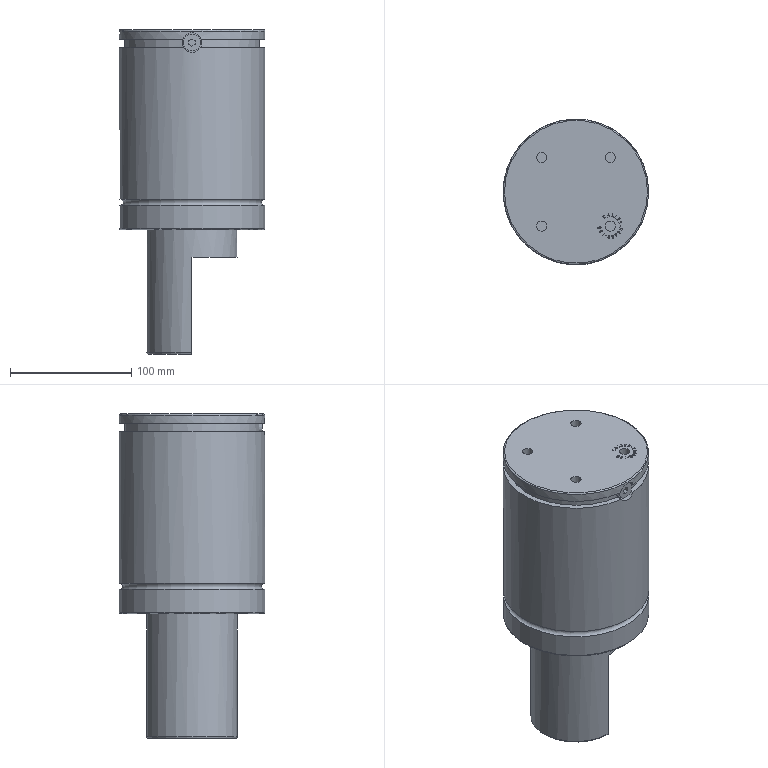Part | NX | features DG 2 | 1 solid | 173 faces | box 120.2 x 120.2 x 268 mm | volume 2131476 mm3 | plane 132 | spline 23 | cylinder 12 | torus 4 | cone 2 | commonest cylinder face diameters 8.4 x4 120.2 x3 6.6 x1 14 x1 16.4 x1 75 x1